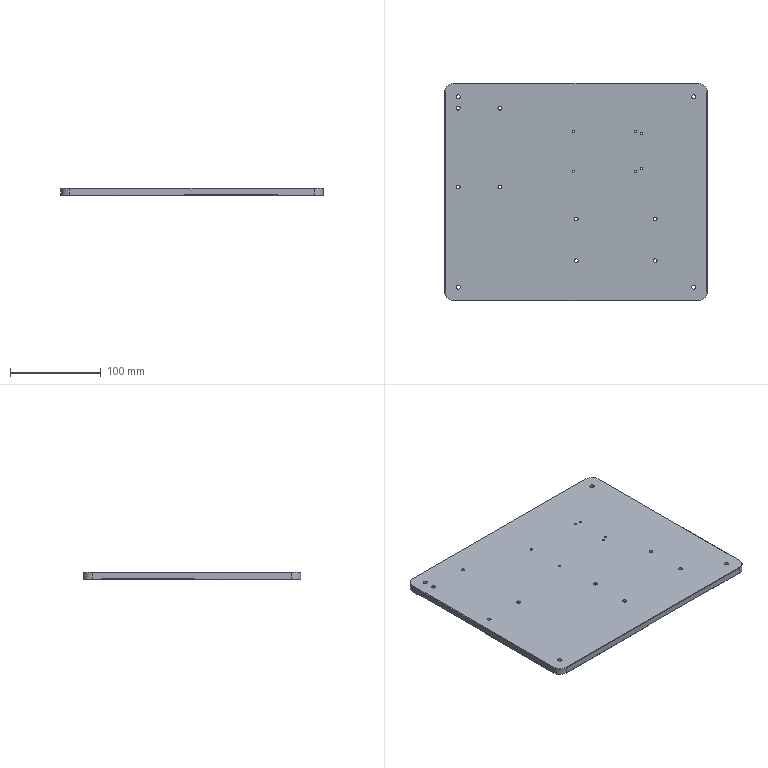Part | 1 solid | 70 faces | box 290 x 240 x 8 mm | volume 535390 mm3 | cylinder 32 | plane 30 | cone 8 | commonest cylinder face diameters 4.2 x8 2.5 x6 2 x4 4.5 x4 8 x4 20 x4